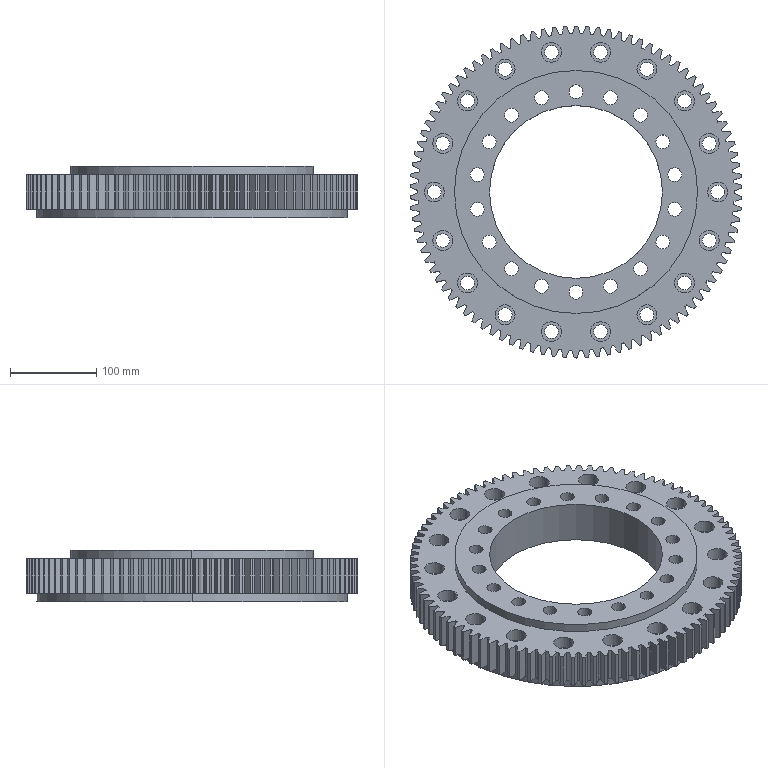Part | SolidWorks | features ICE 4, HoleWzd 2, CirPattern 1, Extrusion 1 | 1 solid | 570 faces | box 383.896 x 384 x 60 mm | volume 3397645 mm3 | cylinder 341 | spline 188 | plane 41 | commonest cylinder face diameters 366 x95 384 x94 16 x72 23 x72 281 x4 200 x2